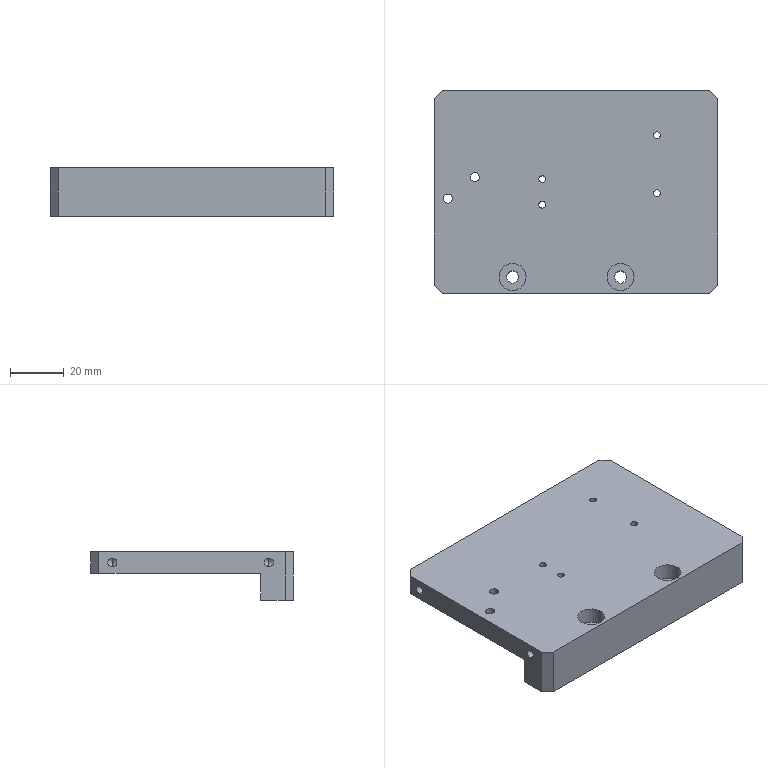Part | STEP file | 1 solid | 56 faces | box 105 x 75 x 18 mm | volume 73147 mm3 | cylinder 32 | plane 16 | cone 8 | commonest cylinder face diameters 2.5 x8 3.3 x8 3.4 x4 4.5 x4 7 x4 10 x4